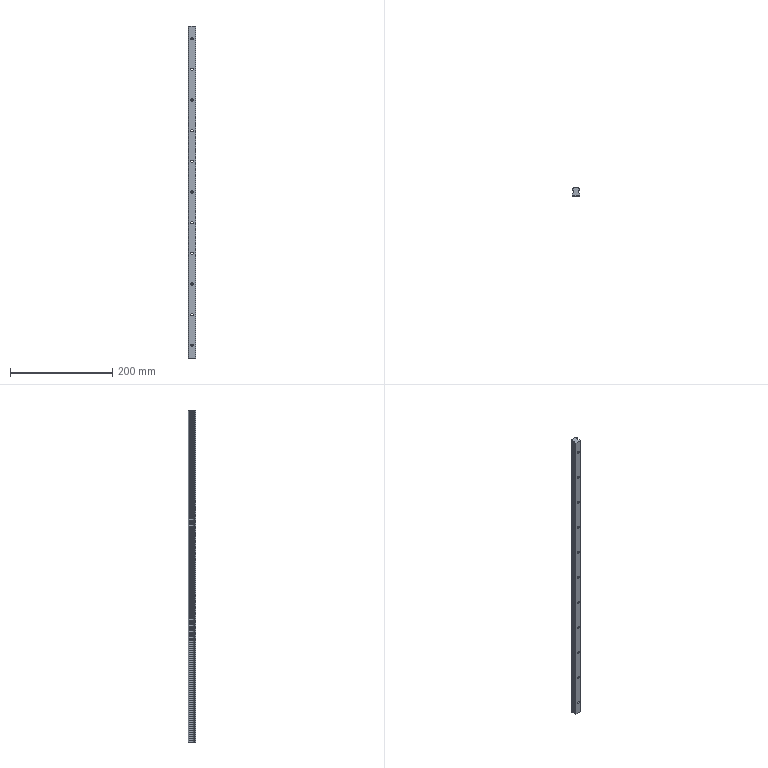Part | SolidWorks | features MoveFace 2, BaseBody 1, LPattern 1 | 1 solid | 91 faces | box 15 x 15 x 650 mm | volume 119721 mm3 | cylinder 58 | plane 33 | commonest cylinder face diameters 4.5 x22 7.5 x22 0.8 x8 3.24 x4 2 x2